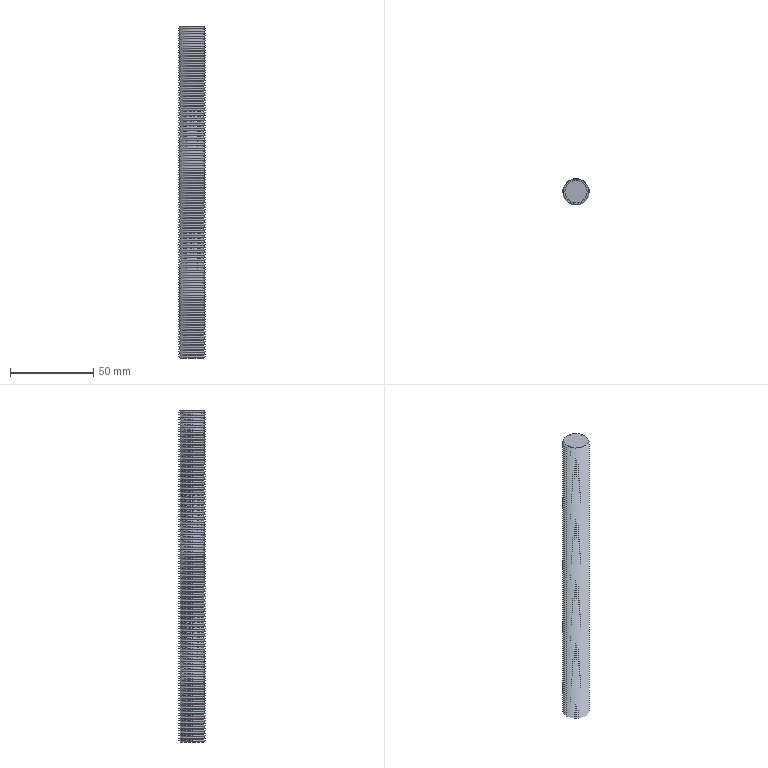Part | STEP file | GB/T 15389 M16×200_M16×200 | 1 solid | 802 faces | box 16 x 16 x 200 mm | volume 34031 mm3 | cone 534 | cylinder 266 | plane 2 | commonest cylinder face diameters 16 x266